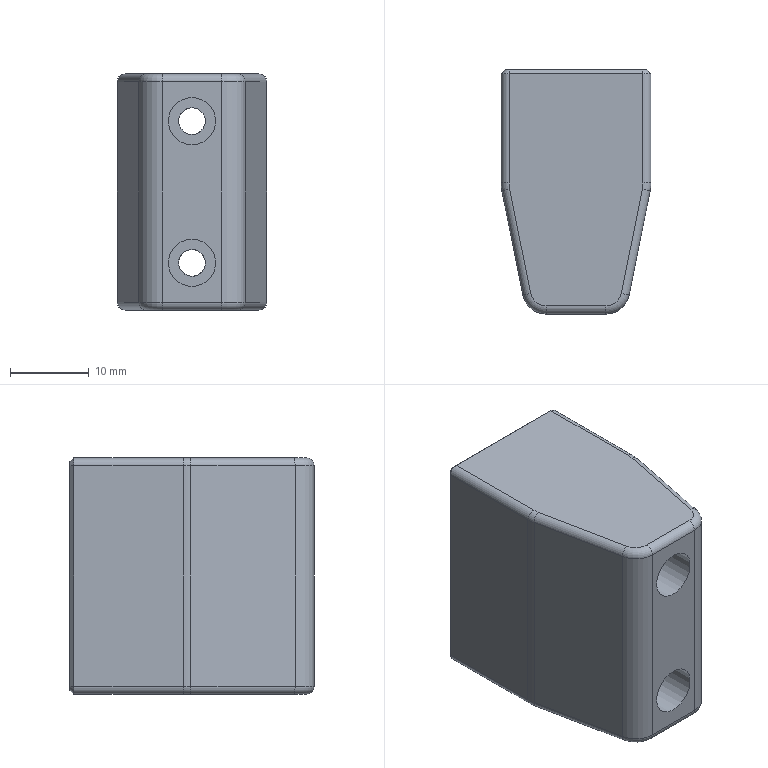Part | 1 solid | 48 faces | box 19 x 31 x 30 mm | volume 14727 mm3 | cylinder 20 | plane 14 | torus 8 | cone 6 | commonest cylinder face diameters 2 x10 6 x4 3 x2 3.4 x2 10 x2
STEP:
#1=CARTESIAN_POINT('',(8.5,0.,0.5));
#2=VERTEX_POINT('',#1);
#3=CARTESIAN_POINT('',(8.5,-0.5,0.));
#4=VERTEX_POINT('',#3);
#5=CARTESIAN_POINT('',(8.5,0.,0.5));
#6=DIRECTION('',(0.,-0.7071,-0.7071));
#7=VECTOR('',#6,1000.);
#8=LINE('',#5,#7);
#9=EDGE_CURVE('',#2,#4,#8,.T.);
#10=ORIENTED_EDGE('',*,*,#9,.T.);
#11=CARTESIAN_POINT('',(-8.5,-0.5,0.));
#12=VERTEX_POINT('',#11);
#13=CARTESIAN_POINT('',(8.5,-0.5,0.));
#14=DIRECTION('',(1.,0.,0.));
#15=VECTOR('',#14,1000.);
#16=LINE('',#13,#15);
#17=EDGE_CURVE('',#12,#4,#16,.T.);
#18=ORIENTED_EDGE('',*,*,#17,.F.);
#19=CARTESIAN_POINT('',(-8.5,0.,0.5));
#20=VERTEX_POINT('',#19);
#21=CARTESIAN_POINT('',(-8.5,-0.5,0.));
#22=DIRECTION('',(0.,0.7071,0.7071));
#23=VECTOR('',#22,1000.);
#24=LINE('',#21,#23);
#25=EDGE_CURVE('',#12,#20,#24,.T.);
#26=ORIENTED_EDGE('',*,*,#25,.T.);
#27=CARTESIAN_POINT('',(-8.5,0.,0.5));
#28=DIRECTION('',(-1.,0.,0.));
#29=VECTOR('',#28,1000.);
#30=LINE('',#27,#29);
#31=EDGE_CURVE('',#2,#20,#30,.T.);
#32=ORIENTED_EDGE('',*,*,#31,.F.);
#33=EDGE_LOOP('',(#10,#18,#26,#32));
#34=FACE_BOUND('',#33,.T.);
#35=CARTESIAN_POINT('',(12.5,0.,0.5));
#36=DIRECTION('',(0.,0.7071,-0.7071));
#37=DIRECTION('',(1.,0.,0.));
#38=AXIS2_PLACEMENT_3D('',#35,#36,#37);
#39=PLANE('',#38);
#40=ADVANCED_FACE('',(#34),#39,.T.);
#41=CARTESIAN_POINT('',(-9.5,-0.5,1.));
#42=VERTEX_POINT('',#41);
#43=CARTESIAN_POINT('',(-9.,0.,1.));
#44=VERTEX_POINT('',#43);
#45=CARTESIAN_POINT('',(-9.5,-0.5,1.));
#46=DIRECTION('',(0.7071,0.7071,0.));
#47=VECTOR('',#46,1000.);
#48=LINE('',#45,#47);
#49=EDGE_CURVE('',#42,#44,#48,.T.);
#50=ORIENTED_EDGE('',*,*,#49,.T.);
#51=CARTESIAN_POINT('',(-8.5,0.,1.));
#52=DIRECTION('',(0.,1.,0.));
#53=DIRECTION('',(-1.,0.,0.));
#54=AXIS2_PLACEMENT_3D('',#51,#52,#53);
#55=CIRCLE('',#54,0.5);
#56=EDGE_CURVE('',#20,#44,#55,.T.);
#57=ORIENTED_EDGE('',*,*,#56,.F.);
#58=ORIENTED_EDGE('',*,*,#25,.F.);
#59=CARTESIAN_POINT('',(-8.5,-0.5,1.));
#60=DIRECTION('',(0.,-1.,0.));
#61=DIRECTION('',(0.,0.,1.));
#62=AXIS2_PLACEMENT_3D('',#59,#60,#61);
#63=CIRCLE('',#62,1.);
#64=EDGE_CURVE('',#42,#12,#63,.T.);
#65=ORIENTED_EDGE('',*,*,#64,.F.);
#66=EDGE_LOOP('',(#50,#57,#58,#65));
#67=FACE_BOUND('',#66,.T.);
#68=CARTESIAN_POINT('',(-8.5,0.,1.));
#69=DIRECTION('',(0.,-1.,0.));
#70=DIRECTION('',(0.,0.,-1.));
#71=AXIS2_PLACEMENT_3D('',#68,#69,#70);
#72=CONICAL_SURFACE('',#71,0.5,0.7854);
#73=ADVANCED_FACE('',(#67),#72,.T.);
#74=CARTESIAN_POINT('',(9.,0.,1.));
#75=VERTEX_POINT('',#74);
#76=CARTESIAN_POINT('',(9.5,-0.5,1.));
#77=VERTEX_POINT('',#76);
#78=CARTESIAN_POINT('',(9.,0.,1.));
#79=DIRECTION('',(0.7071,-0.7071,0.));
#80=VECTOR('',#79,1000.);
#81=LINE('',#78,#80);
#82=EDGE_CURVE('',#75,#77,#81,.T.);
#83=ORIENTED_EDGE('',*,*,#82,.T.);
#84=CARTESIAN_POINT('',(8.5,-0.5,1.));
#85=DIRECTION('',(0.,-1.,0.));
#86=DIRECTION('',(0.,0.,1.));
#87=AXIS2_PLACEMENT_3D('',#84,#85,#86);
#88=CIRCLE('',#87,1.);
#89=EDGE_CURVE('',#4,#77,#88,.T.);
#90=ORIENTED_EDGE('',*,*,#89,.F.);
#91=ORIENTED_EDGE('',*,*,#9,.F.);
#92=CARTESIAN_POINT('',(8.5,0.,1.));
#93=DIRECTION('',(0.,1.,0.));
#94=DIRECTION('',(-1.,0.,0.));
#95=AXIS2_PLACEMENT_3D('',#92,#93,#94);
#96=CIRCLE('',#95,0.5);
#97=EDGE_CURVE('',#75,#2,#96,.T.);
#98=ORIENTED_EDGE('',*,*,#97,.F.);
#99=EDGE_LOOP('',(#83,#90,#91,#98));
#100=FACE_BOUND('',#99,.T.);
#101=CARTESIAN_POINT('',(8.5,0.,1.));
#102=DIRECTION('',(0.,-1.,0.));
#103=DIRECTION('',(0.,0.,-1.));
#104=AXIS2_PLACEMENT_3D('',#101,#102,#103);
#105=CONICAL_SURFACE('',#104,0.5,0.7854);
#106=ADVANCED_FACE('',(#100),#105,.T.);
#107=CARTESIAN_POINT('',(-9.5,-0.5,29.));
#108=VERTEX_POINT('',#107);
#109=CARTESIAN_POINT('',(-9.,0.,29.));
#110=VERTEX_POINT('',#109);
#111=CARTESIAN_POINT('',(-9.5,-0.5,29.));
#112=DIRECTION('',(0.7071,0.7071,0.));
#113=VECTOR('',#112,1000.);
#114=LINE('',#111,#113);
#115=EDGE_CURVE('',#108,#110,#114,.T.);
#116=ORIENTED_EDGE('',*,*,#115,.T.);
#117=CARTESIAN_POINT('',(-9.,0.,29.));
#118=DIRECTION('',(0.,0.,1.));
#119=VECTOR('',#118,1000.);
#120=LINE('',#117,#119);
#121=EDGE_CURVE('',#44,#110,#120,.T.);
#122=ORIENTED_EDGE('',*,*,#121,.F.);
#123=ORIENTED_EDGE('',*,*,#49,.F.);
#124=CARTESIAN_POINT('',(-9.5,-0.5,1.));
#125=DIRECTION('',(0.,0.,-1.));
#126=VECTOR('',#125,1000.);
#127=LINE('',#124,#126);
#128=EDGE_CURVE('',#108,#42,#127,.T.);
#129=ORIENTED_EDGE('',*,*,#128,.F.);
#130=EDGE_LOOP('',(#116,#122,#123,#129));
#131=FACE_BOUND('',#130,.T.);
#132=CARTESIAN_POINT('',(-9.,0.,0.));
#133=DIRECTION('',(-0.7071,0.7071,0.));
#134=DIRECTION('',(0.,0.,-1.));
#135=AXIS2_PLACEMENT_3D('',#132,#133,#134);
#136=PLANE('',#135);
#137=ADVANCED_FACE('',(#131),#136,.T.);
#138=CARTESIAN_POINT('',(9.,0.,29.));
#139=VERTEX_POINT('',#138);
#140=CARTESIAN_POINT('',(9.5,-0.5,29.));
#141=VERTEX_POINT('',#140);
#142=CARTESIAN_POINT('',(9.,0.,29.));
#143=DIRECTION('',(0.7071,-0.7071,0.));
#144=VECTOR('',#143,1000.);
#145=LINE('',#142,#144);
#146=EDGE_CURVE('',#139,#141,#145,.T.);
#147=ORIENTED_EDGE('',*,*,#146,.T.);
#148=CARTESIAN_POINT('',(9.5,-0.5,29.));
#149=DIRECTION('',(0.,0.,1.));
#150=VECTOR('',#149,1000.);
#151=LINE('',#148,#150);
#152=EDGE_CURVE('',#77,#141,#151,.T.);
#153=ORIENTED_EDGE('',*,*,#152,.F.);
#154=ORIENTED_EDGE('',*,*,#82,.F.);
#155=CARTESIAN_POINT('',(9.,0.,1.));
#156=DIRECTION('',(0.,0.,-1.));
#157=VECTOR('',#156,1000.);
#158=LINE('',#155,#157);
#159=EDGE_CURVE('',#139,#75,#158,.T.);
#160=ORIENTED_EDGE('',*,*,#159,.F.);
#161=EDGE_LOOP('',(#147,#153,#154,#160));
#162=FACE_BOUND('',#161,.T.);
#163=CARTESIAN_POINT('',(9.5,-0.5,-30.));
#164=DIRECTION('',(0.7071,0.7071,0.));
#165=DIRECTION('',(0.,0.,-1.));
#166=AXIS2_PLACEMENT_3D('',#163,#164,#165);
#167=PLANE('',#166);
#168=ADVANCED_FACE('',(#162),#167,.T.);
#169=CARTESIAN_POINT('',(-8.5,-0.5,30.));
#170=VERTEX_POINT('',#169);
#171=CARTESIAN_POINT('',(-8.5,0.,29.5));
#172=VERTEX_POINT('',#171);
#173=CARTESIAN_POINT('',(-8.5,-0.5,30.));
#174=DIRECTION('',(0.,0.7071,-0.7071));
#175=VECTOR('',#174,1000.);
#176=LINE('',#173,#175);
#177=EDGE_CURVE('',#170,#172,#176,.T.);
#178=ORIENTED_EDGE('',*,*,#177,.T.);
#179=CARTESIAN_POINT('',(-8.5,0.,29.));
#180=DIRECTION('',(0.,1.,0.));
#181=DIRECTION('',(-1.,0.,0.));
#182=AXIS2_PLACEMENT_3D('',#179,#180,#181);
#183=CIRCLE('',#182,0.5);
#184=EDGE_CURVE('',#110,#172,#183,.T.);
#185=ORIENTED_EDGE('',*,*,#184,.F.);
#186=ORIENTED_EDGE('',*,*,#115,.F.);
#187=CARTESIAN_POINT('',(-8.5,-0.5,29.));
#188=DIRECTION('',(0.,-1.,0.));
#189=DIRECTION('',(0.,0.,1.));
#190=AXIS2_PLACEMENT_3D('',#187,#188,#189);
#191=CIRCLE('',#190,1.);
#192=EDGE_CURVE('',#170,#108,#191,.T.);
#193=ORIENTED_EDGE('',*,*,#192,.F.);
#194=EDGE_LOOP('',(#178,#185,#186,#193));
#195=FACE_BOUND('',#194,.T.);
#196=CARTESIAN_POINT('',(-8.5,0.,29.));
#197=DIRECTION('',(0.,-1.,0.));
#198=DIRECTION('',(0.,0.,-1.));
#199=AXIS2_PLACEMENT_3D('',#196,#197,#198);
#200=CONICAL_SURFACE('',#199,0.5,0.7854);
#201=ADVANCED_FACE('',(#195),#200,.T.);
#202=CARTESIAN_POINT('',(8.5,0.,29.5));
#203=VERTEX_POINT('',#202);
#204=CARTESIAN_POINT('',(8.5,-0.5,30.));
#205=VERTEX_POINT('',#204);
#206=CARTESIAN_POINT('',(8.5,0.,29.5));
#207=DIRECTION('',(0.,-0.7071,0.7071));
#208=VECTOR('',#207,1000.);
#209=LINE('',#206,#208);
#210=EDGE_CURVE('',#203,#205,#209,.T.);
#211=ORIENTED_EDGE('',*,*,#210,.T.);
#212=CARTESIAN_POINT('',(8.5,-0.5,29.));
#213=DIRECTION('',(0.,-1.,0.));
#214=DIRECTION('',(0.,0.,1.));
#215=AXIS2_PLACEMENT_3D('',#212,#213,#214);
#216=CIRCLE('',#215,1.);
#217=EDGE_CURVE('',#141,#205,#216,.T.);
#218=ORIENTED_EDGE('',*,*,#217,.F.);
#219=ORIENTED_EDGE('',*,*,#146,.F.);
#220=CARTESIAN_POINT('',(8.5,0.,29.));
#221=DIRECTION('',(0.,1.,0.));
#222=DIRECTION('',(-1.,0.,0.));
#223=AXIS2_PLACEMENT_3D('',#220,#221,#222);
#224=CIRCLE('',#223,0.5);
#225=EDGE_CURVE('',#203,#139,#224,.T.);
#226=ORIENTED_EDGE('',*,*,#225,.F.);
#227=EDGE_LOOP('',(#211,#218,#219,#226));
#228=FACE_BOUND('',#227,.T.);
#229=CARTESIAN_POINT('',(8.5,0.,29.));
#230=DIRECTION('',(0.,-1.,0.));
#231=DIRECTION('',(0.,0.,-1.));
#232=AXIS2_PLACEMENT_3D('',#229,#230,#231);
#233=CONICAL_SURFACE('',#232,0.5,0.7854);
#234=ADVANCED_FACE('',(#228),#233,.T.);
#235=ORIENTED_EDGE('',*,*,#177,.F.);
#236=CARTESIAN_POINT('',(0.,-0.5,30.));
#237=DIRECTION('',(-1.,0.,0.));
#238=VECTOR('',#237,1000.);
#239=LINE('',#236,#238);
#240=EDGE_CURVE('',#205,#170,#239,.T.);
#241=ORIENTED_EDGE('',*,*,#240,.F.);
#242=ORIENTED_EDGE('',*,*,#210,.F.);
#243=CARTESIAN_POINT('',(12.5,0.,29.5));
#244=DIRECTION('',(1.,0.,0.));
#245=VECTOR('',#244,1000.);
#246=LINE('',#243,#245);
#247=EDGE_CURVE('',#172,#203,#246,.T.);
#248=ORIENTED_EDGE('',*,*,#247,.F.);
#249=EDGE_LOOP('',(#235,#241,#242,#248));
#250=FACE_BOUND('',#249,.T.);
#251=CARTESIAN_POINT('',(0.,-0.5,30.));
#252=DIRECTION('',(0.,-0.7071,-0.7071));
#253=DIRECTION('',(-1.,0.,0.));
#254=AXIS2_PLACEMENT_3D('',#251,#252,#253);
#255=PLANE('',#254);
#256=ADVANCED_FACE('',(#250),#255,.F.);
#257=CARTESIAN_POINT('',(0.,-16.,9.));
#258=VERTEX_POINT('',#257);
#259=CARTESIAN_POINT('',(0.,-16.,6.));
#260=DIRECTION('',(0.,-1.,0.));
#261=DIRECTION('',(0.,0.,1.));
#262=AXIS2_PLACEMENT_3D('',#259,#260,#261);
#263=CIRCLE('',#262,3.);
#264=EDGE_CURVE('',#258,#258,#263,.T.);
#265=ORIENTED_EDGE('',*,*,#264,.T.);
#266=EDGE_LOOP('',(#265));
#267=FACE_BOUND('',#266,.T.);
#268=CARTESIAN_POINT('',(0.,-16.,7.7));
#269=VERTEX_POINT('',#268);
#270=CARTESIAN_POINT('',(0.,-16.,6.));
#271=DIRECTION('',(0.,-1.,0.));
#272=DIRECTION('',(0.,0.,1.));
#273=AXIS2_PLACEMENT_3D('',#270,#271,#272);
#274=CIRCLE('',#273,1.7);
#275=EDGE_CURVE('',#269,#269,#274,.T.);
#276=ORIENTED_EDGE('',*,*,#275,.F.);
#277=EDGE_LOOP('',(#276));
#278=FACE_BOUND('',#277,.T.);
#279=CARTESIAN_POINT('',(1.7,-16.,24.));
#280=DIRECTION('',(0.,1.,0.));
#281=DIRECTION('',(0.,0.,1.));
#282=AXIS2_PLACEMENT_3D('',#279,#280,#281);
#283=PLANE('',#282);
#284=ADVANCED_FACE('',(#267,#278),#283,.F.);
#285=CARTESIAN_POINT('',(0.,-16.,21.));
#286=VERTEX_POINT('',#285);
#287=CARTESIAN_POINT('',(0.,-16.,24.));
#288=DIRECTION('',(0.,-1.,0.));
#289=DIRECTION('',(0.,0.,-1.));
#290=AXIS2_PLACEMENT_3D('',#287,#288,#289);
#291=CIRCLE('',#290,3.);
#292=EDGE_CURVE('',#286,#286,#291,.T.);
#293=ORIENTED_EDGE('',*,*,#292,.T.);
#294=EDGE_LOOP('',(#293));
#295=FACE_BOUND('',#294,.T.);
#296=CARTESIAN_POINT('',(0.,-16.,22.3));
#297=VERTEX_POINT('',#296);
#298=CARTESIAN_POINT('',(0.,-16.,24.));
#299=DIRECTION('',(0.,-1.,0.));
#300=DIRECTION('',(0.,0.,-1.));
#301=AXIS2_PLACEMENT_3D('',#298,#299,#300);
#302=CIRCLE('',#301,1.7);
#303=EDGE_CURVE('',#297,#297,#302,.T.);
#304=ORIENTED_EDGE('',*,*,#303,.F.);
#305=EDGE_LOOP('',(#304));
#306=FACE_BOUND('',#305,.T.);
#307=CARTESIAN_POINT('',(1.7,-16.,24.));
#308=DIRECTION('',(0.,1.,0.));
#309=DIRECTION('',(0.,0.,1.));
#310=AXIS2_PLACEMENT_3D('',#307,#308,#309);
#311=PLANE('',#310);
#312=ADVANCED_FACE('',(#295,#306),#311,.F.);
#313=CARTESIAN_POINT('',(8.5,-14.381,30.));
#314=VERTEX_POINT('',#313);
#315=CARTESIAN_POINT('',(9.5,-14.381,29.));
#316=VERTEX_POINT('',#315);
#317=CARTESIAN_POINT('',(8.5,-14.381,29.));
#318=DIRECTION('',(0.,1.,0.));
#319=DIRECTION('',(0.,0.,1.));
#320=AXIS2_PLACEMENT_3D('',#317,#318,#319);
#321=CIRCLE('',#320,1.);
#322=EDGE_CURVE('',#314,#316,#321,.T.);
#323=ORIENTED_EDGE('',*,*,#322,.F.);
#324=CARTESIAN_POINT('',(8.421,-15.172,30.));
#325=VERTEX_POINT('',#324);
#326=CARTESIAN_POINT('',(4.5,-14.381,30.));
#327=DIRECTION('',(0.,0.,-1.));
#328=DIRECTION('',(1.,0.,0.));
#329=AXIS2_PLACEMENT_3D('',#326,#327,#328);
#330=CIRCLE('',#329,4.);
#331=EDGE_CURVE('',#314,#325,#330,.T.);
#332=ORIENTED_EDGE('',*,*,#331,.T.);
#333=CARTESIAN_POINT('',(9.401,-15.369,29.));
#334=VERTEX_POINT('',#333);
#335=CARTESIAN_POINT('',(8.421,-15.172,29.));
#336=DIRECTION('',(-0.1976,-0.9803,0.));
#337=DIRECTION('',(0.9803,-0.1976,0.));
#338=AXIS2_PLACEMENT_3D('',#335,#336,#337);
#339=CIRCLE('',#338,1.);
#340=EDGE_CURVE('',#334,#325,#339,.T.);
#341=ORIENTED_EDGE('',*,*,#340,.F.);
#342=CARTESIAN_POINT('',(4.5,-14.381,29.));
#343=DIRECTION('',(0.,0.,1.));
#344=DIRECTION('',(1.,0.,0.));
#345=AXIS2_PLACEMENT_3D('',#342,#343,#344);
#346=CIRCLE('',#345,5.);
#347=EDGE_CURVE('',#334,#316,#346,.T.);
#348=ORIENTED_EDGE('',*,*,#347,.T.);
#349=EDGE_LOOP('',(#323,#332,#341,#348));
#350=FACE_BOUND('',#349,.T.);
#351=CARTESIAN_POINT('',(4.5,-14.381,29.));
#352=DIRECTION('',(0.,0.,1.));
#353=DIRECTION('',(1.,0.,0.));
#354=AXIS2_PLACEMENT_3D('',#351,#352,#353);
#355=TOROIDAL_SURFACE('',#354,4.,1.);
#356=ADVANCED_FACE('',(#350),#355,.T.);
#357=CARTESIAN_POINT('',(9.401,-15.369,1.));
#358=VERTEX_POINT('',#357);
#359=CARTESIAN_POINT('',(9.5,-14.381,1.));
#360=VERTEX_POINT('',#359);
#361=CARTESIAN_POINT('',(4.5,-14.381,1.));
#362=DIRECTION('',(0.,0.,1.));
#363=DIRECTION('',(1.,0.,0.));
#364=AXIS2_PLACEMENT_3D('',#361,#362,#363);
#365=CIRCLE('',#364,5.);
#366=EDGE_CURVE('',#358,#360,#365,.T.);
#367=ORIENTED_EDGE('',*,*,#366,.T.);
#368=CARTESIAN_POINT('',(9.5,-14.381,1.));
#369=DIRECTION('',(0.,0.,-1.));
#370=VECTOR('',#369,1000.);
#371=LINE('',#368,#370);
#372=EDGE_CURVE('',#316,#360,#371,.T.);
#373=ORIENTED_EDGE('',*,*,#372,.F.);
#374=ORIENTED_EDGE('',*,*,#347,.F.);
#375=CARTESIAN_POINT('',(9.401,-15.369,29.));
#376=DIRECTION('',(0.,0.,1.));
#377=VECTOR('',#376,1000.);
#378=LINE('',#375,#377);
#379=EDGE_CURVE('',#358,#334,#378,.T.);
#380=ORIENTED_EDGE('',*,*,#379,.F.);
#381=EDGE_LOOP('',(#367,#373,#374,#380));
#382=FACE_BOUND('',#381,.T.);
#383=CARTESIAN_POINT('',(4.5,-14.381,0.));
#384=DIRECTION('',(0.,0.,-1.));
#385=DIRECTION('',(-1.,0.,0.));
#386=AXIS2_PLACEMENT_3D('',#383,#384,#385);
#387=CYLINDRICAL_SURFACE('',#386,5.);
#388=ADVANCED_FACE('',(#382),#387,.T.);
#389=CARTESIAN_POINT('',(8.421,-15.172,0.));
#390=VERTEX_POINT('',#389);
#391=CARTESIAN_POINT('',(8.5,-14.381,0.));
#392=VERTEX_POINT('',#391);
#393=CARTESIAN_POINT('',(4.5,-14.381,0.));
#394=DIRECTION('',(0.,0.,1.));
#395=DIRECTION('',(1.,0.,0.));
#396=AXIS2_PLACEMENT_3D('',#393,#394,#395);
#397=CIRCLE('',#396,4.);
#398=EDGE_CURVE('',#390,#392,#397,.T.);
#399=ORIENTED_EDGE('',*,*,#398,.T.);
#400=CARTESIAN_POINT('',(8.5,-14.381,1.));
#401=DIRECTION('',(0.,1.,0.));
#402=DIRECTION('',(0.,0.,1.));
#403=AXIS2_PLACEMENT_3D('',#400,#401,#402);
#404=CIRCLE('',#403,1.);
#405=EDGE_CURVE('',#360,#392,#404,.T.);
#406=ORIENTED_EDGE('',*,*,#405,.F.);
#407=ORIENTED_EDGE('',*,*,#366,.F.);
#408=CARTESIAN_POINT('',(8.421,-15.172,1.));
#409=DIRECTION('',(-0.1976,-0.9803,0.));
#410=DIRECTION('',(0.9803,-0.1976,0.));
#411=AXIS2_PLACEMENT_3D('',#408,#409,#410);
#412=CIRCLE('',#411,1.);
#413=EDGE_CURVE('',#390,#358,#412,.T.);
#414=ORIENTED_EDGE('',*,*,#413,.F.);
#415=EDGE_LOOP('',(#399,#406,#407,#414));
#416=FACE_BOUND('',#415,.T.);
#417=CARTESIAN_POINT('',(4.5,-14.381,1.));
#418=DIRECTION('',(0.,0.,1.));
#419=DIRECTION('',(1.,0.,0.));
#420=AXIS2_PLACEMENT_3D('',#417,#418,#419);
#421=TOROIDAL_SURFACE('',#420,4.,1.);
#422=ADVANCED_FACE('',(#416),#421,.T.);
#423=CARTESIAN_POINT('',(-9.5,-14.381,29.));
#424=VERTEX_POINT('',#423);
#425=CARTESIAN_POINT('',(-8.5,-14.381,30.));
#426=VERTEX_POINT('',#425);
#427=CARTESIAN_POINT('',(-8.5,-14.381,29.));
#428=DIRECTION('',(0.,1.,0.));
#429=DIRECTION('',(0.,0.,1.));
#430=AXIS2_PLACEMENT_3D('',#427,#428,#429);
#431=CIRCLE('',#430,1.);
#432=EDGE_CURVE('',#424,#426,#431,.T.);
#433=ORIENTED_EDGE('',*,*,#432,.F.);
#434=CARTESIAN_POINT('',(-9.401,-15.369,29.));
#435=VERTEX_POINT('',#434);
#436=CARTESIAN_POINT('',(-4.5,-14.381,29.));
#437=DIRECTION('',(0.,0.,1.));
#438=DIRECTION('',(1.,0.,0.));
#439=AXIS2_PLACEMENT_3D('',#436,#437,#438);
#440=CIRCLE('',#439,5.);
#441=EDGE_CURVE('',#424,#435,#440,.T.);
#442=ORIENTED_EDGE('',*,*,#441,.T.);
#443=CARTESIAN_POINT('',(-8.421,-15.172,30.));
#444=VERTEX_POINT('',#443);
#445=CARTESIAN_POINT('',(-8.421,-15.172,29.));
#446=DIRECTION('',(0.1976,-0.9803,0.));
#447=DIRECTION('',(0.9803,0.1976,0.));
#448=AXIS2_PLACEMENT_3D('',#445,#446,#447);
#449=CIRCLE('',#448,1.);
#450=EDGE_CURVE('',#444,#435,#449,.T.);
#451=ORIENTED_EDGE('',*,*,#450,.F.);
#452=CARTESIAN_POINT('',(-4.5,-14.381,30.));
#453=DIRECTION('',(0.,0.,-1.));
#454=DIRECTION('',(1.,0.,0.));
#455=AXIS2_PLACEMENT_3D('',#452,#453,#454);
#456=CIRCLE('',#455,4.);
#457=EDGE_CURVE('',#444,#426,#456,.T.);
#458=ORIENTED_EDGE('',*,*,#457,.T.);
#459=EDGE_LOOP('',(#433,#442,#451,#458));
#460=FACE_BOUND('',#459,.T.);
#461=CARTESIAN_POINT('',(-4.5,-14.381,29.));
#462=DIRECTION('',(0.,0.,1.));
#463=DIRECTION('',(1.,0.,0.));
#464=AXIS2_PLACEMENT_3D('',#461,#462,#463);
#465=TOROIDAL_SURFACE('',#464,4.,1.);
#466=ADVANCED_FACE('',(#460),#465,.T.);
#467=CARTESIAN_POINT('',(-9.5,-14.381,1.));
#468=VERTEX_POINT('',#467);
#469=CARTESIAN_POINT('',(-9.401,-15.369,1.));
#470=VERTEX_POINT('',#469);
#471=CARTESIAN_POINT('',(-4.5,-14.381,1.));
#472=DIRECTION('',(0.,0.,1.));
#473=DIRECTION('',(1.,0.,0.));
#474=AXIS2_PLACEMENT_3D('',#471,#472,#473);
#475=CIRCLE('',#474,5.);
#476=EDGE_CURVE('',#468,#470,#475,.T.);
#477=ORIENTED_EDGE('',*,*,#476,.T.);
#478=CARTESIAN_POINT('',(-9.401,-15.369,1.));
#479=DIRECTION('',(0.,0.,-1.));
#480=VECTOR('',#479,1000.);
#481=LINE('',#478,#480);
#482=EDGE_CURVE('',#435,#470,#481,.T.);
#483=ORIENTED_EDGE('',*,*,#482,.F.);
#484=ORIENTED_EDGE('',*,*,#441,.F.);
#485=CARTESIAN_POINT('',(-9.5,-14.381,29.));
#486=DIRECTION('',(0.,0.,1.));
#487=VECTOR('',#486,1000.);
#488=LINE('',#485,#487);
#489=EDGE_CURVE('',#468,#424,#488,.T.);
#490=ORIENTED_EDGE('',*,*,#489,.F.);
#491=EDGE_LOOP('',(#477,#483,#484,#490));
#492=FACE_BOUND('',#491,.T.);
#493=CARTESIAN_POINT('',(-4.5,-14.381,-30.));
#494=DIRECTION('',(0.,0.,-1.));
#495=DIRECTION('',(-1.,0.,0.));
#496=AXIS2_PLACEMENT_3D('',#493,#494,#495);
#497=CYLINDRICAL_SURFACE('',#496,5.);
#498=ADVANCED_FACE('',(#492),#497,.T.);
#499=CARTESIAN_POINT('',(-8.5,-14.381,0.));
#500=VERTEX_POINT('',#499);
#501=CARTESIAN_POINT('',(-8.421,-15.172,0.));
#502=VERTEX_POINT('',#501);
#503=CARTESIAN_POINT('',(-4.5,-14.381,0.));
#504=DIRECTION('',(0.,0.,1.));
#505=DIRECTION('',(1.,0.,0.));
#506=AXIS2_PLACEMENT_3D('',#503,#504,#505);
#507=CIRCLE('',#506,4.);
#508=EDGE_CURVE('',#500,#502,#507,.T.);
#509=ORIENTED_EDGE('',*,*,#508,.T.);
#510=CARTESIAN_POINT('',(-8.421,-15.172,1.));
#511=DIRECTION('',(0.1976,-0.9803,0.));
#512=DIRECTION('',(0.9803,0.1976,0.));
#513=AXIS2_PLACEMENT_3D('',#510,#511,#512);
#514=CIRCLE('',#513,1.);
#515=EDGE_CURVE('',#470,#502,#514,.T.);
#516=ORIENTED_EDGE('',*,*,#515,.F.);
#517=ORIENTED_EDGE('',*,*,#476,.F.);
#518=CARTESIAN_POINT('',(-8.5,-14.381,1.));
#519=DIRECTION('',(0.,1.,0.));
#520=DIRECTION('',(0.,0.,1.));
#521=AXIS2_PLACEMENT_3D('',#518,#519,#520);
#522=CIRCLE('',#521,1.);
#523=EDGE_CURVE('',#500,#468,#522,.T.);
#524=ORIENTED_EDGE('',*,*,#523,.F.);
#525=EDGE_LOOP('',(#509,#516,#517,#524));
#526=FACE_BOUND('',#525,.T.);
#527=CARTESIAN_POINT('',(-4.5,-14.381,1.));
#528=DIRECTION('',(0.,0.,1.));
#529=DIRECTION('',(1.,0.,0.));
#530=AXIS2_PLACEMENT_3D('',#527,#528,#529);
#531=TOROIDAL_SURFACE('',#530,4.,1.);
#532=ADVANCED_FACE('',(#526),#531,.T.);
#533=CARTESIAN_POINT('',(-6.735,-28.593,1.));
#534=VERTEX_POINT('',#533);
#535=CARTESIAN_POINT('',(-6.735,-28.593,1.));
#536=DIRECTION('',(0.1976,-0.9803,0.));
#537=VECTOR('',#536,1000.);
#538=LINE('',#535,#537);
#539=EDGE_CURVE('',#470,#534,#538,.T.);
#540=ORIENTED_EDGE('',*,*,#539,.F.);
#541=ORIENTED_EDGE('',*,*,#515,.T.);
#542=CARTESIAN_POINT('',(-5.755,-28.395,0.));
#543=VERTEX_POINT('',#542);
#544=CARTESIAN_POINT('',(-8.52,-14.682,0.));
#545=DIRECTION('',(-0.1976,0.9803,0.));
#546=VECTOR('',#545,1000.);
#547=LINE('',#544,#546);
#548=EDGE_CURVE('',#543,#502,#547,.T.);
#549=ORIENTED_EDGE('',*,*,#548,.F.);
#550=CARTESIAN_POINT('',(-5.755,-28.395,1.));
#551=DIRECTION('',(-0.1976,0.9803,0.));
#552=DIRECTION('',(-0.9803,-0.1976,0.));
#553=AXIS2_PLACEMENT_3D('',#550,#551,#552);
#554=CIRCLE('',#553,1.);
#555=EDGE_CURVE('',#543,#534,#554,.T.);
#556=ORIENTED_EDGE('',*,*,#555,.T.);
#557=EDGE_LOOP('',(#540,#541,#549,#556));
#558=FACE_BOUND('',#557,.T.);
#559=CARTESIAN_POINT('',(-11.52,0.1976,1.));
#560=DIRECTION('',(-0.1976,0.9803,0.));
#561=DIRECTION('',(-0.9803,-0.1976,0.));
#562=AXIS2_PLACEMENT_3D('',#559,#560,#561);
#563=CYLINDRICAL_SURFACE('',#562,1.);
#564=ADVANCED_FACE('',(#558),#563,.T.);
#565=CARTESIAN_POINT('',(-3.794,-30.,0.));
#566=VERTEX_POINT('',#565);
#567=CARTESIAN_POINT('',(-3.794,-31.,1.));
#568=VERTEX_POINT('',#567);
#569=CARTESIAN_POINT('',(-3.794,-30.,1.));
#570=DIRECTION('',(-1.,0.,0.));
#571=DIRECTION('',(0.,0.,1.));
#572=AXIS2_PLACEMENT_3D('',#569,#570,#571);
#573=CIRCLE('',#572,1.);
#574=EDGE_CURVE('',#566,#568,#573,.T.);
#575=ORIENTED_EDGE('',*,*,#574,.T.);
#576=CARTESIAN_POINT('',(-3.794,-28.,1.));
#577=DIRECTION('',(0.,0.,1.));
#578=DIRECTION('',(1.,0.,0.));
#579=AXIS2_PLACEMENT_3D('',#576,#577,#578);
#580=CIRCLE('',#579,3.);
#581=EDGE_CURVE('',#534,#568,#580,.T.);
#582=ORIENTED_EDGE('',*,*,#581,.F.);
#583=ORIENTED_EDGE('',*,*,#555,.F.);
#584=CARTESIAN_POINT('',(-3.794,-28.,0.));
#585=DIRECTION('',(0.,0.,-1.));
#586=DIRECTION('',(1.,0.,0.));
#587=AXIS2_PLACEMENT_3D('',#584,#585,#586);
#588=CIRCLE('',#587,2.);
#589=EDGE_CURVE('',#566,#543,#588,.T.);
#590=ORIENTED_EDGE('',*,*,#589,.F.);
#591=EDGE_LOOP('',(#575,#582,#583,#590));
#592=FACE_BOUND('',#591,.T.);
#593=CARTESIAN_POINT('',(-3.794,-28.,1.));
#594=DIRECTION('',(0.,0.,1.));
#595=DIRECTION('',(1.,0.,0.));
#596=AXIS2_PLACEMENT_3D('',#593,#594,#595);
#597=TOROIDAL_SURFACE('',#596,2.,1.);
#598=ADVANCED_FACE('',(#592),#597,.T.);
#599=CARTESIAN_POINT('',(-9.5,0.,1.));
#600=DIRECTION('',(0.,-1.,0.));
#601=VECTOR('',#600,1000.);
#602=LINE('',#599,#601);
#603=EDGE_CURVE('',#42,#468,#602,.T.);
#604=ORIENTED_EDGE('',*,*,#603,.F.);
#605=ORIENTED_EDGE('',*,*,#64,.T.);
#606=CARTESIAN_POINT('',(-8.5,0.,0.));
#607=DIRECTION('',(0.,1.,0.));
#608=VECTOR('',#607,1000.);
#609=LINE('',#606,#608);
#610=EDGE_CURVE('',#500,#12,#609,.T.);
#611=ORIENTED_EDGE('',*,*,#610,.F.);
#612=ORIENTED_EDGE('',*,*,#523,.T.);
#613=EDGE_LOOP('',(#604,#605,#611,#612));
#614=FACE_BOUND('',#613,.T.);
#615=CARTESIAN_POINT('',(-8.5,0.,1.));
#616=DIRECTION('',(0.,1.,0.));
#617=DIRECTION('',(-1.,0.,0.));
#618=AXIS2_PLACEMENT_3D('',#615,#616,#617);
#619=CYLINDRICAL_SURFACE('',#618,1.);
#620=ADVANCED_FACE('',(#614),#619,.T.);
#621=CARTESIAN_POINT('',(3.794,-30.,0.));
#622=VERTEX_POINT('',#621);
#623=CARTESIAN_POINT('',(3.794,-31.,1.));
#624=VERTEX_POINT('',#623);
#625=CARTESIAN_POINT('',(3.794,-30.,1.));
#626=DIRECTION('',(-1.,0.,0.));
#627=DIRECTION('',(0.,0.,1.));
#628=AXIS2_PLACEMENT_3D('',#625,#626,#627);
#629=CIRCLE('',#628,1.);
#630=EDGE_CURVE('',#622,#624,#629,.T.);
#631=ORIENTED_EDGE('',*,*,#630,.T.);
#632=CARTESIAN_POINT('',(3.794,-31.,1.));
#633=DIRECTION('',(1.,0.,0.));
#634=VECTOR('',#633,1000.);
#635=LINE('',#632,#634);
#636=EDGE_CURVE('',#568,#624,#635,.T.);
#637=ORIENTED_EDGE('',*,*,#636,.F.);
#638=ORIENTED_EDGE('',*,*,#574,.F.);
#639=CARTESIAN_POINT('',(-3.794,-30.,0.));
#640=DIRECTION('',(-1.,0.,0.));
#641=VECTOR('',#640,1000.);
#642=LINE('',#639,#641);
#643=EDGE_CURVE('',#622,#566,#642,.T.);
#644=ORIENTED_EDGE('',*,*,#643,.F.);
#645=EDGE_LOOP('',(#631,#637,#638,#644));
#646=FACE_BOUND('',#645,.T.);
#647=CARTESIAN_POINT('',(-6.25,-30.,1.));
#648=DIRECTION('',(-1.,0.,0.));
#649=DIRECTION('',(0.,0.,1.));
#650=AXIS2_PLACEMENT_3D('',#647,#648,#649);
#651=CYLINDRICAL_SURFACE('',#650,1.);
#652=ADVANCED_FACE('',(#646),#651,.T.);
#653=CARTESIAN_POINT('',(5.755,-28.395,0.));
#654=VERTEX_POINT('',#653);
#655=CARTESIAN_POINT('',(6.735,-28.593,1.));
#656=VERTEX_POINT('',#655);
#657=CARTESIAN_POINT('',(5.755,-28.395,1.));
#658=DIRECTION('',(-0.1976,-0.9803,0.));
#659=DIRECTION('',(0.9803,-0.1976,0.));
#660=AXIS2_PLACEMENT_3D('',#657,#658,#659);
#661=CIRCLE('',#660,1.);
#662=EDGE_CURVE('',#654,#656,#661,.T.);
#663=ORIENTED_EDGE('',*,*,#662,.T.);
#664=CARTESIAN_POINT('',(3.794,-28.,1.));
#665=DIRECTION('',(0.,0.,1.));
#666=DIRECTION('',(1.,0.,0.));
#667=AXIS2_PLACEMENT_3D('',#664,#665,#666);
#668=CIRCLE('',#667,3.);
#669=EDGE_CURVE('',#624,#656,#668,.T.);
#670=ORIENTED_EDGE('',*,*,#669,.F.);
#671=ORIENTED_EDGE('',*,*,#630,.F.);
#672=CARTESIAN_POINT('',(3.794,-28.,0.));
#673=DIRECTION('',(0.,0.,-1.));
#674=DIRECTION('',(1.,0.,0.));
#675=AXIS2_PLACEMENT_3D('',#672,#673,#674);
#676=CIRCLE('',#675,2.);
#677=EDGE_CURVE('',#654,#622,#676,.T.);
#678=ORIENTED_EDGE('',*,*,#677,.F.);
#679=EDGE_LOOP('',(#663,#670,#671,#678));
#680=FACE_BOUND('',#679,.T.);
#681=CARTESIAN_POINT('',(3.794,-28.,1.));
#682=DIRECTION('',(0.,0.,1.));
#683=DIRECTION('',(1.,0.,0.));
#684=AXIS2_PLACEMENT_3D('',#681,#682,#683);
#685=TOROIDAL_SURFACE('',#684,2.,1.);
#686=ADVANCED_FACE('',(#680),#685,.T.);
#687=CARTESIAN_POINT('',(5.755,-28.395,0.));
#688=DIRECTION('',(-0.1976,-0.9803,0.));
#689=VECTOR('',#688,1000.);
#690=LINE('',#687,#689);
#691=EDGE_CURVE('',#390,#654,#690,.T.);
#692=ORIENTED_EDGE('',*,*,#691,.F.);
#693=ORIENTED_EDGE('',*,*,#413,.T.);
#694=CARTESIAN_POINT('',(9.5,-14.88,1.));
#695=DIRECTION('',(0.1976,0.9803,0.));
#696=VECTOR('',#695,1000.);
#697=LINE('',#694,#696);
#698=EDGE_CURVE('',#656,#358,#697,.T.);
#699=ORIENTED_EDGE('',*,*,#698,.F.);
#700=ORIENTED_EDGE('',*,*,#662,.F.);
#701=EDGE_LOOP('',(#692,#693,#699,#700));
#702=FACE_BOUND('',#701,.T.);
#703=CARTESIAN_POINT('',(5.27,-30.802,1.));
#704=DIRECTION('',(-0.1976,-0.9803,0.));
#705=DIRECTION('',(0.9803,-0.1976,0.));
#706=AXIS2_PLACEMENT_3D('',#703,#704,#705);
#707=CYLINDRICAL_SURFACE('',#706,1.);
#708=ADVANCED_FACE('',(#702),#707,.T.);
#709=CARTESIAN_POINT('',(8.5,0.,0.));
#710=DIRECTION('',(0.,-1.,0.));
#711=VECTOR('',#710,1000.);
#712=LINE('',#709,#711);
#713=EDGE_CURVE('',#4,#392,#712,.T.);
#714=ORIENTED_EDGE('',*,*,#713,.F.);
#715=ORIENTED_EDGE('',*,*,#89,.T.);
#716=CARTESIAN_POINT('',(9.5,0.,1.));
#717=DIRECTION('',(0.,1.,0.));
#718=VECTOR('',#717,1000.);
#719=LINE('',#716,#718);
#720=EDGE_CURVE('',#360,#77,#719,.T.);
#721=ORIENTED_EDGE('',*,*,#720,.F.);
#722=ORIENTED_EDGE('',*,*,#405,.T.);
#723=EDGE_LOOP('',(#714,#715,#721,#722));
#724=FACE_BOUND('',#723,.T.);
#725=CARTESIAN_POINT('',(8.5,0.,1.));
#726=DIRECTION('',(0.,-1.,0.));
#727=DIRECTION('',(1.,0.,0.));
#728=AXIS2_PLACEMENT_3D('',#725,#726,#727);
#729=CYLINDRICAL_SURFACE('',#728,1.);
#730=ADVANCED_FACE('',(#724),#729,.T.);
#731=CARTESIAN_POINT('',(-5.755,-28.395,30.));
#732=VERTEX_POINT('',#731);
#733=CARTESIAN_POINT('',(-11.031,-2.224,30.));
#734=DIRECTION('',(0.1976,-0.9803,0.));
#735=VECTOR('',#734,1000.);
#736=LINE('',#733,#735);
#737=EDGE_CURVE('',#444,#732,#736,.T.);
#738=ORIENTED_EDGE('',*,*,#737,.F.);
#739=ORIENTED_EDGE('',*,*,#450,.T.);
#740=CARTESIAN_POINT('',(-6.735,-28.593,29.));
#741=VERTEX_POINT('',#740);
#742=CARTESIAN_POINT('',(-12.5,0.,29.));
#743=DIRECTION('',(-0.1976,0.9803,0.));
#744=VECTOR('',#743,1000.);
#745=LINE('',#742,#744);
#746=EDGE_CURVE('',#741,#435,#745,.T.);
#747=ORIENTED_EDGE('',*,*,#746,.F.);
#748=CARTESIAN_POINT('',(-5.755,-28.395,29.));
#749=DIRECTION('',(-0.1976,0.9803,0.));
#750=DIRECTION('',(-0.9803,-0.1976,0.));
#751=AXIS2_PLACEMENT_3D('',#748,#749,#750);
#752=CIRCLE('',#751,1.);
#753=EDGE_CURVE('',#741,#732,#752,.T.);
#754=ORIENTED_EDGE('',*,*,#753,.T.);
#755=EDGE_LOOP('',(#738,#739,#747,#754));
#756=FACE_BOUND('',#755,.T.);
#757=CARTESIAN_POINT('',(-11.031,-2.224,29.));
#758=DIRECTION('',(0.1976,-0.9803,0.));
#759=DIRECTION('',(0.9803,0.1976,0.));
#760=AXIS2_PLACEMENT_3D('',#757,#758,#759);
#761=CYLINDRICAL_SURFACE('',#760,1.);
#762=ADVANCED_FACE('',(#756),#761,.T.);
#763=CARTESIAN_POINT('',(-3.794,-31.,29.));
#764=VERTEX_POINT('',#763);
#765=CARTESIAN_POINT('',(-3.794,-30.,30.));
#766=VERTEX_POINT('',#765);
#767=CARTESIAN_POINT('',(-3.794,-30.,29.));
#768=DIRECTION('',(-1.,0.,0.));
#769=DIRECTION('',(0.,0.,1.));
#770=AXIS2_PLACEMENT_3D('',#767,#768,#769);
#771=CIRCLE('',#770,1.);
#772=EDGE_CURVE('',#764,#766,#771,.T.);
#773=ORIENTED_EDGE('',*,*,#772,.T.);
#774=CARTESIAN_POINT('',(-3.794,-28.,30.));
#775=DIRECTION('',(0.,0.,1.));
#776=DIRECTION('',(1.,0.,0.));
#777=AXIS2_PLACEMENT_3D('',#774,#775,#776);
#778=CIRCLE('',#777,2.);
#779=EDGE_CURVE('',#732,#766,#778,.T.);
#780=ORIENTED_EDGE('',*,*,#779,.F.);
#781=ORIENTED_EDGE('',*,*,#753,.F.);
#782=CARTESIAN_POINT('',(-3.794,-28.,29.));
#783=DIRECTION('',(0.,0.,-1.));
#784=DIRECTION('',(1.,0.,0.));
#785=AXIS2_PLACEMENT_3D('',#782,#783,#784);
#786=CIRCLE('',#785,3.);
#787=EDGE_CURVE('',#764,#741,#786,.T.);
#788=ORIENTED_EDGE('',*,*,#787,.F.);
#789=EDGE_LOOP('',(#773,#780,#781,#788));
#790=FACE_BOUND('',#789,.T.);
#791=CARTESIAN_POINT('',(-3.794,-28.,29.));
#792=DIRECTION('',(0.,0.,1.));
#793=DIRECTION('',(1.,0.,0.));
#794=AXIS2_PLACEMENT_3D('',#791,#792,#793);
#795=TOROIDAL_SURFACE('',#794,2.,1.);
#796=ADVANCED_FACE('',(#790),#795,.T.);
#797=CARTESIAN_POINT('',(-8.5,-14.88,30.));
#798=DIRECTION('',(0.,-1.,0.));
#799=VECTOR('',#798,1000.);
#800=LINE('',#797,#799);
#801=EDGE_CURVE('',#170,#426,#800,.T.);
#802=ORIENTED_EDGE('',*,*,#801,.F.);
#803=ORIENTED_EDGE('',*,*,#192,.T.);
#804=CARTESIAN_POINT('',(-9.5,0.,29.));
#805=DIRECTION('',(0.,1.,0.));
#806=VECTOR('',#805,1000.);
#807=LINE('',#804,#806);
#808=EDGE_CURVE('',#424,#108,#807,.T.);
#809=ORIENTED_EDGE('',*,*,#808,.F.);
#810=ORIENTED_EDGE('',*,*,#432,.T.);
#811=EDGE_LOOP('',(#802,#803,#809,#810));
#812=FACE_BOUND('',#811,.T.);
#813=CARTESIAN_POINT('',(-8.5,0.,29.));
#814=DIRECTION('',(0.,-1.,0.));
#815=DIRECTION('',(1.,0.,0.));
#816=AXIS2_PLACEMENT_3D('',#813,#814,#815);
#817=CYLINDRICAL_SURFACE('',#816,1.);
#818=ADVANCED_FACE('',(#812),#817,.T.);
#819=CARTESIAN_POINT('',(3.794,-31.,29.));
#820=VERTEX_POINT('',#819);
#821=CARTESIAN_POINT('',(3.794,-30.,30.));
#822=VERTEX_POINT('',#821);
#823=CARTESIAN_POINT('',(3.794,-30.,29.));
#824=DIRECTION('',(-1.,0.,0.));
#825=DIRECTION('',(0.,0.,1.));
#826=AXIS2_PLACEMENT_3D('',#823,#824,#825);
#827=CIRCLE('',#826,1.);
#828=EDGE_CURVE('',#820,#822,#827,.T.);
#829=ORIENTED_EDGE('',*,*,#828,.T.);
#830=CARTESIAN_POINT('',(0.,-30.,30.));
#831=DIRECTION('',(1.,0.,0.));
#832=VECTOR('',#831,1000.);
#833=LINE('',#830,#832);
#834=EDGE_CURVE('',#766,#822,#833,.T.);
#835=ORIENTED_EDGE('',*,*,#834,.F.);
#836=ORIENTED_EDGE('',*,*,#772,.F.);
#837=CARTESIAN_POINT('',(-6.25,-31.,29.));
#838=DIRECTION('',(-1.,0.,0.));
#839=VECTOR('',#838,1000.);
#840=LINE('',#837,#839);
#841=EDGE_CURVE('',#820,#764,#840,.T.);
#842=ORIENTED_EDGE('',*,*,#841,.F.);
#843=EDGE_LOOP('',(#829,#835,#836,#842));
#844=FACE_BOUND('',#843,.T.);
#845=CARTESIAN_POINT('',(0.,-30.,29.));
#846=DIRECTION('',(1.,0.,0.));
#847=DIRECTION('',(0.,0.,-1.));
#848=AXIS2_PLACEMENT_3D('',#845,#846,#847);
#849=CYLINDRICAL_SURFACE('',#848,1.);
#850=ADVANCED_FACE('',(#844),#849,.T.);
#851=CARTESIAN_POINT('',(6.735,-28.593,29.));
#852=VERTEX_POINT('',#851);
#853=CARTESIAN_POINT('',(5.755,-28.395,30.));
#854=VERTEX_POINT('',#853);
#855=CARTESIAN_POINT('',(5.755,-28.395,29.));
#856=DIRECTION('',(-0.1976,-0.9803,0.));
#857=DIRECTION('',(0.9803,-0.1976,0.));
#858=AXIS2_PLACEMENT_3D('',#855,#856,#857);
#859=CIRCLE('',#858,1.);
#860=EDGE_CURVE('',#852,#854,#859,.T.);
#861=ORIENTED_EDGE('',*,*,#860,.T.);
#862=CARTESIAN_POINT('',(3.794,-28.,30.));
#863=DIRECTION('',(0.,0.,1.));
#864=DIRECTION('',(1.,0.,0.));
#865=AXIS2_PLACEMENT_3D('',#862,#863,#864);
#866=CIRCLE('',#865,2.);
#867=EDGE_CURVE('',#822,#854,#866,.T.);
#868=ORIENTED_EDGE('',*,*,#867,.F.);
#869=ORIENTED_EDGE('',*,*,#828,.F.);
#870=CARTESIAN_POINT('',(3.794,-28.,29.));
#871=DIRECTION('',(0.,0.,-1.));
#872=DIRECTION('',(1.,0.,0.));
#873=AXIS2_PLACEMENT_3D('',#870,#871,#872);
#874=CIRCLE('',#873,3.);
#875=EDGE_CURVE('',#852,#820,#874,.T.);
#876=ORIENTED_EDGE('',*,*,#875,.F.);
#877=EDGE_LOOP('',(#861,#868,#869,#876));
#878=FACE_BOUND('',#877,.T.);
#879=CARTESIAN_POINT('',(3.794,-28.,29.));
#880=DIRECTION('',(0.,0.,1.));
#881=DIRECTION('',(1.,0.,0.));
#882=AXIS2_PLACEMENT_3D('',#879,#880,#881);
#883=TOROIDAL_SURFACE('',#882,2.,1.);
#884=ADVANCED_FACE('',(#878),#883,.T.);
#885=CARTESIAN_POINT('',(6.25,-31.,29.));
#886=DIRECTION('',(-0.1976,-0.9803,0.));
#887=VECTOR('',#886,1000.);
#888=LINE('',#885,#887);
#889=EDGE_CURVE('',#334,#852,#888,.T.);
#890=ORIENTED_EDGE('',*,*,#889,.F.);
#891=ORIENTED_EDGE('',*,*,#340,.T.);
#892=CARTESIAN_POINT('',(11.031,-2.224,30.));
#893=DIRECTION('',(0.1976,0.9803,0.));
#894=VECTOR('',#893,1000.);
#895=LINE('',#892,#894);
#896=EDGE_CURVE('',#854,#325,#895,.T.);
#897=ORIENTED_EDGE('',*,*,#896,.F.);
#898=ORIENTED_EDGE('',*,*,#860,.F.);
#899=EDGE_LOOP('',(#890,#891,#897,#898));
#900=FACE_BOUND('',#899,.T.);
#901=CARTESIAN_POINT('',(11.031,-2.224,29.));
#902=DIRECTION('',(0.1976,0.9803,0.));
#903=DIRECTION('',(-0.9803,0.1976,0.));
#904=AXIS2_PLACEMENT_3D('',#901,#902,#903);
#905=CYLINDRICAL_SURFACE('',#904,1.);
#906=ADVANCED_FACE('',(#900),#905,.T.);
#907=CARTESIAN_POINT('',(9.5,-14.88,29.));
#908=DIRECTION('',(0.,-1.,0.));
#909=VECTOR('',#908,1000.);
#910=LINE('',#907,#909);
#911=EDGE_CURVE('',#141,#316,#910,.T.);
#912=ORIENTED_EDGE('',*,*,#911,.F.);
#913=ORIENTED_EDGE('',*,*,#217,.T.);
#914=CARTESIAN_POINT('',(8.5,0.,30.));
#915=DIRECTION('',(0.,1.,0.));
#916=VECTOR('',#915,1000.);
#917=LINE('',#914,#916);
#918=EDGE_CURVE('',#314,#205,#917,.T.);
#919=ORIENTED_EDGE('',*,*,#918,.F.);
#920=ORIENTED_EDGE('',*,*,#322,.T.);
#921=EDGE_LOOP('',(#912,#913,#919,#920));
#922=FACE_BOUND('',#921,.T.);
#923=CARTESIAN_POINT('',(8.5,0.,29.));
#924=DIRECTION('',(0.,1.,0.));
#925=DIRECTION('',(-1.,0.,0.));
#926=AXIS2_PLACEMENT_3D('',#923,#924,#925);
#927=CYLINDRICAL_SURFACE('',#926,1.);
#928=ADVANCED_FACE('',(#922),#927,.T.);
#929=CARTESIAN_POINT('',(-3.794,-31.,0.));
#930=DIRECTION('',(0.,0.,-1.));
#931=VECTOR('',#930,1000.);
#932=LINE('',#929,#931);
#933=EDGE_CURVE('',#764,#568,#932,.T.);
#934=ORIENTED_EDGE('',*,*,#933,.F.);
#935=ORIENTED_EDGE('',*,*,#787,.T.);
#936=CARTESIAN_POINT('',(-6.735,-28.593,0.));
#937=DIRECTION('',(0.,0.,1.));
#938=VECTOR('',#937,1000.);
#939=LINE('',#936,#938);
#940=EDGE_CURVE('',#534,#741,#939,.T.);
#941=ORIENTED_EDGE('',*,*,#940,.F.);
#942=ORIENTED_EDGE('',*,*,#581,.T.);
#943=EDGE_LOOP('',(#934,#935,#941,#942));
#944=FACE_BOUND('',#943,.T.);
#945=CARTESIAN_POINT('',(-3.794,-28.,0.));
#946=DIRECTION('',(0.,0.,1.));
#947=DIRECTION('',(1.,0.,0.));
#948=AXIS2_PLACEMENT_3D('',#945,#946,#947);
#949=CYLINDRICAL_SURFACE('',#948,3.);
#950=ADVANCED_FACE('',(#944),#949,.T.);
#951=CARTESIAN_POINT('',(6.735,-28.593,0.));
#952=DIRECTION('',(0.,0.,-1.));
#953=VECTOR('',#952,1000.);
#954=LINE('',#951,#953);
#955=EDGE_CURVE('',#852,#656,#954,.T.);
#956=ORIENTED_EDGE('',*,*,#955,.F.);
#957=ORIENTED_EDGE('',*,*,#875,.T.);
#958=CARTESIAN_POINT('',(3.794,-31.,0.));
#959=DIRECTION('',(0.,0.,1.));
#960=VECTOR('',#959,1000.);
#961=LINE('',#958,#960);
#962=EDGE_CURVE('',#624,#820,#961,.T.);
#963=ORIENTED_EDGE('',*,*,#962,.F.);
#964=ORIENTED_EDGE('',*,*,#669,.T.);
#965=EDGE_LOOP('',(#956,#957,#963,#964));
#966=FACE_BOUND('',#965,.T.);
#967=CARTESIAN_POINT('',(3.794,-28.,0.));
#968=DIRECTION('',(0.,0.,1.));
#969=DIRECTION('',(1.,0.,0.));
#970=AXIS2_PLACEMENT_3D('',#967,#968,#969);
#971=CYLINDRICAL_SURFACE('',#970,3.);
#972=ADVANCED_FACE('',(#966),#971,.T.);
#973=ORIENTED_EDGE('',*,*,#808,.T.);
#974=ORIENTED_EDGE('',*,*,#128,.T.);
#975=ORIENTED_EDGE('',*,*,#603,.T.);
#976=ORIENTED_EDGE('',*,*,#489,.T.);
#977=EDGE_LOOP('',(#973,#974,#975,#976));
#978=FACE_BOUND('',#977,.T.);
#979=CARTESIAN_POINT('',(-9.5,0.,-30.));
#980=DIRECTION('',(1.,0.,0.));
#981=DIRECTION('',(0.,1.,0.));
#982=AXIS2_PLACEMENT_3D('',#979,#980,#981);
#983=PLANE('',#982);
#984=ADVANCED_FACE('',(#978),#983,.F.);
#985=ORIENTED_EDGE('',*,*,#720,.T.);
#986=ORIENTED_EDGE('',*,*,#152,.T.);
#987=ORIENTED_EDGE('',*,*,#911,.T.);
#988=ORIENTED_EDGE('',*,*,#372,.T.);
#989=EDGE_LOOP('',(#985,#986,#987,#988));
#990=FACE_BOUND('',#989,.T.);
#991=CARTESIAN_POINT('',(9.5,0.,-30.));
#992=DIRECTION('',(-1.,0.,0.));
#993=DIRECTION('',(0.,-1.,0.));
#994=AXIS2_PLACEMENT_3D('',#991,#992,#993);
#995=PLANE('',#994);
#996=ADVANCED_FACE('',(#990),#995,.F.);
#997=ORIENTED_EDGE('',*,*,#746,.T.);
#998=ORIENTED_EDGE('',*,*,#482,.T.);
#999=ORIENTED_EDGE('',*,*,#539,.T.);
#1000=ORIENTED_EDGE('',*,*,#940,.T.);
#1001=EDGE_LOOP('',(#997,#998,#999,#1000));
#1002=FACE_BOUND('',#1001,.T.);
#1003=CARTESIAN_POINT('',(-12.5,0.,0.));
#1004=DIRECTION('',(-0.9803,-0.1976,0.));
#1005=DIRECTION('',(0.1976,-0.9803,0.));
#1006=AXIS2_PLACEMENT_3D('',#1003,#1004,#1005);
#1007=PLANE('',#1006);
#1008=ADVANCED_FACE('',(#1002),#1007,.T.);
#1009=ORIENTED_EDGE('',*,*,#962,.T.);
#1010=ORIENTED_EDGE('',*,*,#841,.T.);
#1011=ORIENTED_EDGE('',*,*,#933,.T.);
#1012=ORIENTED_EDGE('',*,*,#636,.T.);
#1013=EDGE_LOOP('',(#1009,#1010,#1011,#1012));
#1014=FACE_BOUND('',#1013,.T.);
#1015=CARTESIAN_POINT('',(0.,-31.,21.));
#1016=VERTEX_POINT('',#1015);
#1017=CARTESIAN_POINT('',(0.,-31.,24.));
#1018=DIRECTION('',(0.,-1.,0.));
#1019=DIRECTION('',(0.,0.,-1.));
#1020=AXIS2_PLACEMENT_3D('',#1017,#1018,#1019);
#1021=CIRCLE('',#1020,3.);
#1022=EDGE_CURVE('',#1016,#1016,#1021,.T.);
#1023=ORIENTED_EDGE('',*,*,#1022,.F.);
#1024=EDGE_LOOP('',(#1023));
#1025=FACE_BOUND('',#1024,.T.);
#1026=CARTESIAN_POINT('',(0.,-31.,3.));
#1027=VERTEX_POINT('',#1026);
#1028=CARTESIAN_POINT('',(0.,-31.,6.));
#1029=DIRECTION('',(0.,-1.,0.));
#1030=DIRECTION('',(0.,0.,-1.));
#1031=AXIS2_PLACEMENT_3D('',#1028,#1029,#1030);
#1032=CIRCLE('',#1031,3.);
#1033=EDGE_CURVE('',#1027,#1027,#1032,.T.);
#1034=ORIENTED_EDGE('',*,*,#1033,.F.);
#1035=EDGE_LOOP('',(#1034));
#1036=FACE_BOUND('',#1035,.T.);
#1037=CARTESIAN_POINT('',(-6.25,-31.,0.));
#1038=DIRECTION('',(0.,-1.,0.));
#1039=DIRECTION('',(0.,0.,-1.));
#1040=AXIS2_PLACEMENT_3D('',#1037,#1038,#1039);
#1041=PLANE('',#1040);
#1042=ADVANCED_FACE('',(#1014,#1025,#1036),#1041,.T.);
#1043=ORIENTED_EDGE('',*,*,#698,.T.);
#1044=ORIENTED_EDGE('',*,*,#379,.T.);
#1045=ORIENTED_EDGE('',*,*,#889,.T.);
#1046=ORIENTED_EDGE('',*,*,#955,.T.);
#1047=EDGE_LOOP('',(#1043,#1044,#1045,#1046));
#1048=FACE_BOUND('',#1047,.T.);
#1049=CARTESIAN_POINT('',(6.25,-31.,0.));
#1050=DIRECTION('',(0.9803,-0.1976,0.));
#1051=DIRECTION('',(0.1976,0.9803,0.));
#1052=AXIS2_PLACEMENT_3D('',#1049,#1050,#1051);
#1053=PLANE('',#1052);
#1054=ADVANCED_FACE('',(#1048),#1053,.T.);
#1055=CARTESIAN_POINT('',(-6.,0.,16.5));
#1056=VERTEX_POINT('',#1055);
#1057=CARTESIAN_POINT('',(-6.,0.,15.));
#1058=DIRECTION('',(0.,1.,0.));
#1059=DIRECTION('',(0.,0.,1.));
#1060=AXIS2_PLACEMENT_3D('',#1057,#1058,#1059);
#1061=CIRCLE('',#1060,1.5);
#1062=EDGE_CURVE('',#1056,#1056,#1061,.T.);
#1063=ORIENTED_EDGE('',*,*,#1062,.F.);
#1064=EDGE_LOOP('',(#1063));
#1065=FACE_BOUND('',#1064,.T.);
#1066=CARTESIAN_POINT('',(6.,0.,16.5));
#1067=VERTEX_POINT('',#1066);
#1068=CARTESIAN_POINT('',(6.,0.,15.));
#1069=DIRECTION('',(0.,1.,0.));
#1070=DIRECTION('',(0.,0.,1.));
#1071=AXIS2_PLACEMENT_3D('',#1068,#1069,#1070);
#1072=CIRCLE('',#1071,1.5);
#1073=EDGE_CURVE('',#1067,#1067,#1072,.T.);
#1074=ORIENTED_EDGE('',*,*,#1073,.F.);
#1075=EDGE_LOOP('',(#1074));
#1076=FACE_BOUND('',#1075,.T.);
#1077=CARTESIAN_POINT('',(-1.7,0.,24.));
#1078=VERTEX_POINT('',#1077);
#1079=CARTESIAN_POINT('',(0.,0.,24.));
#1080=DIRECTION('',(0.,1.,0.));
#1081=DIRECTION('',(-1.,0.,0.));
#1082=AXIS2_PLACEMENT_3D('',#1079,#1080,#1081);
#1083=CIRCLE('',#1082,1.7);
#1084=EDGE_CURVE('',#1078,#1078,#1083,.T.);
#1085=ORIENTED_EDGE('',*,*,#1084,.F.);
#1086=EDGE_LOOP('',(#1085));
#1087=FACE_BOUND('',#1086,.T.);
#1088=CARTESIAN_POINT('',(-1.7,0.,6.));
#1089=VERTEX_POINT('',#1088);
#1090=CARTESIAN_POINT('',(0.,0.,6.));
#1091=DIRECTION('',(0.,1.,0.));
#1092=DIRECTION('',(-1.,0.,0.));
#1093=AXIS2_PLACEMENT_3D('',#1090,#1091,#1092);
#1094=CIRCLE('',#1093,1.7);
#1095=EDGE_CURVE('',#1089,#1089,#1094,.T.);
#1096=ORIENTED_EDGE('',*,*,#1095,.F.);
#1097=EDGE_LOOP('',(#1096));
#1098=FACE_BOUND('',#1097,.T.);
#1099=ORIENTED_EDGE('',*,*,#97,.T.);
#1100=ORIENTED_EDGE('',*,*,#31,.T.);
#1101=ORIENTED_EDGE('',*,*,#56,.T.);
#1102=ORIENTED_EDGE('',*,*,#121,.T.);
#1103=ORIENTED_EDGE('',*,*,#184,.T.);
#1104=ORIENTED_EDGE('',*,*,#247,.T.);
#1105=ORIENTED_EDGE('',*,*,#225,.T.);
#1106=ORIENTED_EDGE('',*,*,#159,.T.);
#1107=EDGE_LOOP('',(#1099,#1100,#1101,#1102,#1103,#1104,#1105,#1106));
#1108=FACE_BOUND('',#1107,.T.);
#1109=CARTESIAN_POINT('',(12.5,0.,0.));
#1110=DIRECTION('',(0.,1.,0.));
#1111=DIRECTION('',(-1.,0.,0.));
#1112=AXIS2_PLACEMENT_3D('',#1109,#1110,#1111);
#1113=PLANE('',#1112);
#1114=ADVANCED_FACE('',(#1065,#1076,#1087,#1098,#1108),#1113,.T.);
#1115=ORIENTED_EDGE('',*,*,#918,.T.);
#1116=ORIENTED_EDGE('',*,*,#240,.T.);
#1117=ORIENTED_EDGE('',*,*,#801,.T.);
#1118=ORIENTED_EDGE('',*,*,#457,.F.);
#1119=ORIENTED_EDGE('',*,*,#737,.T.);
#1120=ORIENTED_EDGE('',*,*,#779,.T.);
#1121=ORIENTED_EDGE('',*,*,#834,.T.);
#1122=ORIENTED_EDGE('',*,*,#867,.T.);
#1123=ORIENTED_EDGE('',*,*,#896,.T.);
#1124=ORIENTED_EDGE('',*,*,#331,.F.);
#1125=EDGE_LOOP('',(#1115,#1116,#1117,#1118,#1119,#1120,#1121,#1122,#1123,#1124));
#1126=FACE_BOUND('',#1125,.T.);
#1127=CARTESIAN_POINT('',(0.,0.,30.));
#1128=DIRECTION('',(0.,0.,1.));
#1129=DIRECTION('',(1.,0.,0.));
#1130=AXIS2_PLACEMENT_3D('',#1127,#1128,#1129);
#1131=PLANE('',#1130);
#1132=ADVANCED_FACE('',(#1126),#1131,.T.);
#1133=ORIENTED_EDGE('',*,*,#610,.T.);
#1134=ORIENTED_EDGE('',*,*,#17,.T.);
#1135=ORIENTED_EDGE('',*,*,#713,.T.);
#1136=ORIENTED_EDGE('',*,*,#398,.F.);
#1137=ORIENTED_EDGE('',*,*,#691,.T.);
#1138=ORIENTED_EDGE('',*,*,#677,.T.);
#1139=ORIENTED_EDGE('',*,*,#643,.T.);
#1140=ORIENTED_EDGE('',*,*,#589,.T.);
#1141=ORIENTED_EDGE('',*,*,#548,.T.);
#1142=ORIENTED_EDGE('',*,*,#508,.F.);
#1143=EDGE_LOOP('',(#1133,#1134,#1135,#1136,#1137,#1138,#1139,#1140,#1141,#1142));
#1144=FACE_BOUND('',#1143,.T.);
#1145=CARTESIAN_POINT('',(0.,0.,0.));
#1146=DIRECTION('',(0.,0.,1.));
#1147=DIRECTION('',(1.,0.,0.));
#1148=AXIS2_PLACEMENT_3D('',#1145,#1146,#1147);
#1149=PLANE('',#1148);
#1150=ADVANCED_FACE('',(#1144),#1149,.F.);
#1151=CARTESIAN_POINT('',(-6.,-8.,16.5));
#1152=VERTEX_POINT('',#1151);
#1153=CARTESIAN_POINT('',(-6.,-8.,15.));
#1154=DIRECTION('',(0.,1.,0.));
#1155=DIRECTION('',(0.,0.,1.));
#1156=AXIS2_PLACEMENT_3D('',#1153,#1154,#1155);
#1157=CIRCLE('',#1156,1.5);
#1158=EDGE_CURVE('',#1152,#1152,#1157,.T.);
#1159=ORIENTED_EDGE('',*,*,#1158,.T.);
#1160=EDGE_LOOP('',(#1159));
#1161=FACE_BOUND('',#1160,.T.);
#1162=CARTESIAN_POINT('',(-6.,-8.901,15.));
#1163=VERTEX_POINT('',#1162);
#1164=VERTEX_LOOP('',#1163);
#1165=FACE_BOUND('',#1164,.T.);
#1166=CARTESIAN_POINT('',(-6.,-8.,15.));
#1167=DIRECTION('',(0.,1.,0.));
#1168=DIRECTION('',(0.,0.,1.));
#1169=AXIS2_PLACEMENT_3D('',#1166,#1167,#1168);
#1170=CONICAL_SURFACE('',#1169,1.5,1.03);
#1171=ADVANCED_FACE('',(#1161,#1165),#1170,.F.);
#1172=ORIENTED_EDGE('',*,*,#1158,.F.);
#1173=EDGE_LOOP('',(#1172));
#1174=FACE_BOUND('',#1173,.T.);
#1175=ORIENTED_EDGE('',*,*,#1062,.T.);
#1176=EDGE_LOOP('',(#1175));
#1177=FACE_BOUND('',#1176,.T.);
#1178=CARTESIAN_POINT('',(-6.,0.,15.));
#1179=DIRECTION('',(0.,1.,0.));
#1180=DIRECTION('',(0.,0.,1.));
#1181=AXIS2_PLACEMENT_3D('',#1178,#1179,#1180);
#1182=CYLINDRICAL_SURFACE('',#1181,1.5);
#1183=ADVANCED_FACE('',(#1174,#1177),#1182,.F.);
#1184=CARTESIAN_POINT('',(6.,-8.,16.5));
#1185=VERTEX_POINT('',#1184);
#1186=CARTESIAN_POINT('',(6.,-8.,15.));
#1187=DIRECTION('',(0.,1.,0.));
#1188=DIRECTION('',(0.,0.,1.));
#1189=AXIS2_PLACEMENT_3D('',#1186,#1187,#1188);
#1190=CIRCLE('',#1189,1.5);
#1191=EDGE_CURVE('',#1185,#1185,#1190,.T.);
#1192=ORIENTED_EDGE('',*,*,#1191,.T.);
#1193=EDGE_LOOP('',(#1192));
#1194=FACE_BOUND('',#1193,.T.);
#1195=CARTESIAN_POINT('',(6.,-8.901,15.));
#1196=VERTEX_POINT('',#1195);
#1197=VERTEX_LOOP('',#1196);
#1198=FACE_BOUND('',#1197,.T.);
#1199=CARTESIAN_POINT('',(6.,-8.,15.));
#1200=DIRECTION('',(0.,1.,0.));
#1201=DIRECTION('',(0.,0.,1.));
#1202=AXIS2_PLACEMENT_3D('',#1199,#1200,#1201);
#1203=CONICAL_SURFACE('',#1202,1.5,1.03);
#1204=ADVANCED_FACE('',(#1194,#1198),#1203,.F.);
#1205=ORIENTED_EDGE('',*,*,#1191,.F.);
#1206=EDGE_LOOP('',(#1205));
#1207=FACE_BOUND('',#1206,.T.);
#1208=ORIENTED_EDGE('',*,*,#1073,.T.);
#1209=EDGE_LOOP('',(#1208));
#1210=FACE_BOUND('',#1209,.T.);
#1211=CARTESIAN_POINT('',(6.,0.,15.));
#1212=DIRECTION('',(0.,1.,0.));
#1213=DIRECTION('',(0.,0.,1.));
#1214=AXIS2_PLACEMENT_3D('',#1211,#1212,#1213);
#1215=CYLINDRICAL_SURFACE('',#1214,1.5);
#1216=ADVANCED_FACE('',(#1207,#1210),#1215,.F.);
#1217=ORIENTED_EDGE('',*,*,#303,.T.);
#1218=EDGE_LOOP('',(#1217));
#1219=FACE_BOUND('',#1218,.T.);
#1220=ORIENTED_EDGE('',*,*,#1084,.T.);
#1221=EDGE_LOOP('',(#1220));
#1222=FACE_BOUND('',#1221,.T.);
#1223=CARTESIAN_POINT('',(0.,-31.,24.));
#1224=DIRECTION('',(0.,-1.,0.));
#1225=DIRECTION('',(0.,0.,-1.));
#1226=AXIS2_PLACEMENT_3D('',#1223,#1224,#1225);
#1227=CYLINDRICAL_SURFACE('',#1226,1.7);
#1228=ADVANCED_FACE('',(#1219,#1222),#1227,.F.);
#1229=ORIENTED_EDGE('',*,*,#1022,.T.);
#1230=EDGE_LOOP('',(#1229));
#1231=FACE_BOUND('',#1230,.T.);
#1232=ORIENTED_EDGE('',*,*,#292,.F.);
#1233=EDGE_LOOP('',(#1232));
#1234=FACE_BOUND('',#1233,.T.);
#1235=CARTESIAN_POINT('',(0.,-31.,24.));
#1236=DIRECTION('',(0.,-1.,0.));
#1237=DIRECTION('',(0.,0.,-1.));
#1238=AXIS2_PLACEMENT_3D('',#1235,#1236,#1237);
#1239=CYLINDRICAL_SURFACE('',#1238,3.);
#1240=ADVANCED_FACE('',(#1231,#1234),#1239,.F.);
#1241=ORIENTED_EDGE('',*,*,#275,.T.);
#1242=EDGE_LOOP('',(#1241));
#1243=FACE_BOUND('',#1242,.T.);
#1244=ORIENTED_EDGE('',*,*,#1095,.T.);
#1245=EDGE_LOOP('',(#1244));
#1246=FACE_BOUND('',#1245,.T.);
#1247=CARTESIAN_POINT('',(0.,-31.,6.));
#1248=DIRECTION('',(0.,-1.,0.));
#1249=DIRECTION('',(0.,0.,-1.));
#1250=AXIS2_PLACEMENT_3D('',#1247,#1248,#1249);
#1251=CYLINDRICAL_SURFACE('',#1250,1.7);
#1252=ADVANCED_FACE('',(#1243,#1246),#1251,.F.);
#1253=ORIENTED_EDGE('',*,*,#1033,.T.);
#1254=EDGE_LOOP('',(#1253));
#1255=FACE_BOUND('',#1254,.T.);
#1256=ORIENTED_EDGE('',*,*,#264,.F.);
#1257=EDGE_LOOP('',(#1256));
#1258=FACE_BOUND('',#1257,.T.);
#1259=CARTESIAN_POINT('',(0.,-31.,6.));
#1260=DIRECTION('',(0.,-1.,0.));
#1261=DIRECTION('',(0.,0.,-1.));
#1262=AXIS2_PLACEMENT_3D('',#1259,#1260,#1261);
#1263=CYLINDRICAL_SURFACE('',#1262,3.);
#1264=ADVANCED_FACE('',(#1255,#1258),#1263,.F.);
#1265=CLOSED_SHELL('',(#40,#73,#106,#137,#168,#201,#234,#256,#284,#312,#356,#388,#422,#466,#498,#532,#564,#598,#620,#652,#686,#708,#730,#762,#796,#818,#850,#884,#906,#928,#950,#972,#984,#996,#1008,#1042,#1054,#1114,#1132,#1150,#1171,#1183,#1204,#1216,#1228,#1240,#1252,#1264));
#1266=MANIFOLD_SOLID_BREP('',#1265);
#1267=(LENGTH_UNIT()NAMED_UNIT(*)SI_UNIT(.MILLI.,.METRE.));
#1268=UNCERTAINTY_MEASURE_WITH_UNIT(LENGTH_MEASURE(0.00001),#1267,'','');
#1269=(NAMED_UNIT(*)PLANE_ANGLE_UNIT()SI_UNIT($,.RADIAN.));
#1270=(NAMED_UNIT(*)SI_UNIT($,.STERADIAN.)SOLID_ANGLE_UNIT());
#1271=(GEOMETRIC_REPRESENTATION_CONTEXT(3)GLOBAL_UNCERTAINTY_ASSIGNED_CONTEXT((#1268))GLOBAL_UNIT_ASSIGNED_CONTEXT((#1267,#1269,#1270))REPRESENTATION_CONTEXT('',''));
#1272=ADVANCED_BREP_SHAPE_REPRESENTATION('',(#1266),#1271);